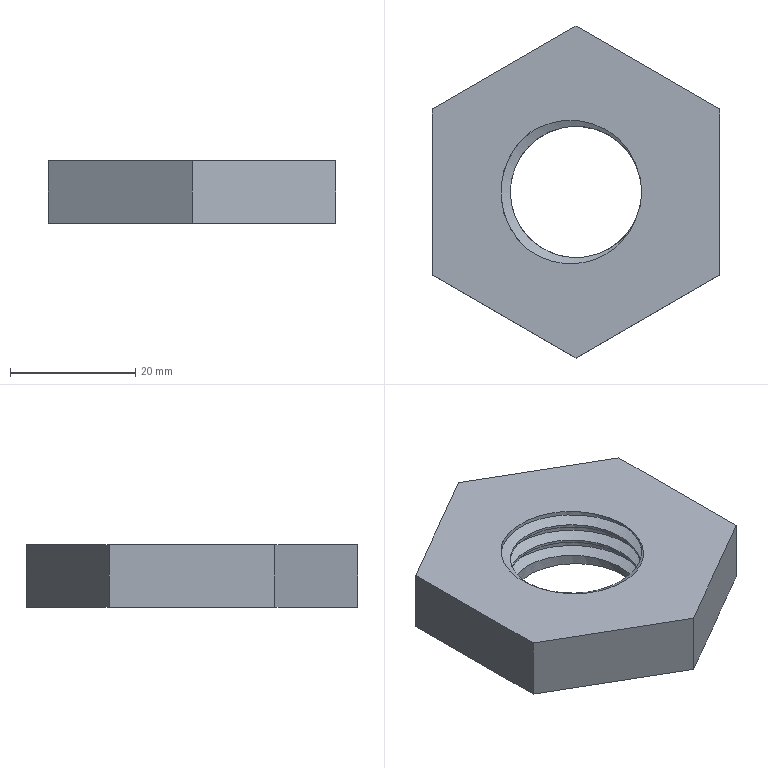Part | NX | features DATUM_CSYS 2, EXTRUDE 1, SKETCH 1, THREADS 1 | 1 solid | 13 faces | box 45.899 x 53 x 10 mm | volume 14258 mm3 | plane 9 | cylinder 2 | spline 2 | commonest cylinder face diameters 21 x1 24 x1
STEP:
#1=CARTESIAN_POINT('',(-9.733,-3.939,-10.));
#2=VERTEX_POINT('',#1);
#3=CARTESIAN_POINT('',(-9.733,-3.939,-7.535));
#4=VERTEX_POINT('',#3);
#5=CARTESIAN_POINT('',(-9.733,-3.939,-10.));
#6=DIRECTION('',(0.,0.,1.));
#7=VECTOR('',#6,1000.);
#8=LINE('',#5,#7);
#9=EDGE_CURVE('',#2,#4,#8,.T.);
#10=ORIENTED_EDGE('',*,*,#9,.F.);
#11=CARTESIAN_POINT('',(-8.724,-5.844,-10.));
#12=VERTEX_POINT('',#11);
#13=CARTESIAN_POINT('',(0.,0.,-10.));
#14=DIRECTION('',(0.,0.,1.));
#15=DIRECTION('',(1.,0.,0.));
#16=AXIS2_PLACEMENT_3D('',#13,#14,#15);
#17=CIRCLE('',#16,10.5);
#18=EDGE_CURVE('',#12,#2,#17,.T.);
#19=ORIENTED_EDGE('',*,*,#18,.F.);
#20=CARTESIAN_POINT('',(9.422,-4.634,0.));
#21=VERTEX_POINT('',#20);
#22=CARTESIAN_POINT('',(-8.724,-5.844,-10.));
#23=CARTESIAN_POINT('',(-7.437,-7.765,-9.895));
#24=CARTESIAN_POINT('',(-3.621,-10.672,-9.688));
#25=CARTESIAN_POINT('',(3.636,-10.678,-9.375));
#26=CARTESIAN_POINT('',(9.381,-6.256,-9.063));
#27=CARTESIAN_POINT('',(11.252,0.747,-8.75));
#28=CARTESIAN_POINT('',(8.472,7.443,-8.438));
#29=CARTESIAN_POINT('',(2.189,11.062,-8.125));
#30=CARTESIAN_POINT('',(-4.998,10.109,-7.813));
#31=CARTESIAN_POINT('',(-10.12,4.976,-7.5));
#32=CARTESIAN_POINT('',(-11.058,-2.214,-7.187));
#33=CARTESIAN_POINT('',(-7.424,-8.489,-6.875));
#34=CARTESIAN_POINT('',(-0.7214,-11.254,-6.562));
#35=CARTESIAN_POINT('',(6.279,-9.367,-6.25));
#36=CARTESIAN_POINT('',(10.684,-3.609,-5.937));
#37=CARTESIAN_POINT('',(10.673,3.64,-5.625));
#38=CARTESIAN_POINT('',(6.252,9.385,-5.312));
#39=CARTESIAN_POINT('',(-0.7512,11.251,-5.));
#40=CARTESIAN_POINT('',(-7.444,8.47,-4.688));
#41=CARTESIAN_POINT('',(-11.062,2.19,-4.375));
#42=CARTESIAN_POINT('',(-10.109,-4.996,-4.063));
#43=CARTESIAN_POINT('',(-4.979,-10.118,-3.75));
#44=CARTESIAN_POINT('',(2.21,-11.058,-3.438));
#45=CARTESIAN_POINT('',(8.486,-7.427,-3.125));
#46=CARTESIAN_POINT('',(11.254,-0.7254,-2.813));
#47=CARTESIAN_POINT('',(9.369,6.276,-2.5));
#48=CARTESIAN_POINT('',(3.611,10.683,-2.187));
#49=CARTESIAN_POINT('',(-3.64,10.673,-1.875));
#50=CARTESIAN_POINT('',(-9.386,6.251,-1.562));
#51=CARTESIAN_POINT('',(-11.252,-0.7548,-1.25));
#52=CARTESIAN_POINT('',(-8.467,-7.447,-0.9373));
#53=CARTESIAN_POINT('',(-2.185,-11.066,-0.625));
#54=CARTESIAN_POINT('',(5.007,-10.095,-0.3119));
#55=CARTESIAN_POINT('',(8.402,-6.709,-0.1051));
#56=CARTESIAN_POINT('',(9.422,-4.634,0.));
#57=B_SPLINE_CURVE_WITH_KNOTS('',3,(#22,#23,#24,#25,#26,#27,#28,#29,#30,#31,#32,#33,#34,#35,#36,#37,#38,#39,#40,#41,#42,#43,#44,#45,#46,#47,#48,#49,#50,#51,#52,#53,#54,#55,#56),.UNSPECIFIED.,.F.,.F.,(4,1,1,1,1,1,1,1,1,1,1,1,1,1,1,1,1,1,1,1,1,1,1,1,1,1,1,1,1,1,1,1,4),(0.,0.006847,0.01369,0.02054,0.02739,0.03423,0.04108,0.04793,0.05477,0.06162,0.06847,0.07531,0.08216,0.08901,0.09585,0.1027,0.1095,0.1164,0.1232,0.1301,0.1369,0.1438,0.1506,0.1575,0.1643,0.1712,0.178,0.1849,0.1917,0.1986,0.2054,0.2123,0.2191),.UNSPECIFIED.);
#58=EDGE_CURVE('',#12,#21,#57,.T.);
#59=ORIENTED_EDGE('',*,*,#58,.T.);
#60=CARTESIAN_POINT('',(9.422,4.634,0.));
#61=VERTEX_POINT('',#60);
#62=CARTESIAN_POINT('',(0.,0.,0.));
#63=DIRECTION('',(0.,0.,1.));
#64=DIRECTION('',(1.,0.,0.));
#65=AXIS2_PLACEMENT_3D('',#62,#63,#64);
#66=CIRCLE('',#65,10.5);
#67=EDGE_CURVE('',#21,#61,#66,.T.);
#68=ORIENTED_EDGE('',*,*,#67,.T.);
#69=CARTESIAN_POINT('',(9.422,4.634,0.));
#70=CARTESIAN_POINT('',(10.191,3.07,-0.07918));
#71=CARTESIAN_POINT('',(10.923,-0.3895,-0.2352));
#72=CARTESIAN_POINT('',(9.443,-5.518,-0.4707));
#73=CARTESIAN_POINT('',(5.696,-9.332,-0.7066));
#74=CARTESIAN_POINT('',(0.6132,-10.918,-0.9414));
#75=CARTESIAN_POINT('',(-4.642,-9.9,-1.178));
#76=CARTESIAN_POINT('',(-8.765,-6.537,-1.412));
#77=CARTESIAN_POINT('',(-10.818,-1.592,-1.648));
#78=CARTESIAN_POINT('',(-10.288,3.703,-1.883));
#79=CARTESIAN_POINT('',(-7.299,8.142,-2.119));
#80=CARTESIAN_POINT('',(-2.586,10.623,-2.354));
#81=CARTESIAN_POINT('',(2.759,10.581,-2.59));
#82=CARTESIAN_POINT('',(7.434,8.017,-2.825));
#83=CARTESIAN_POINT('',(10.345,3.543,-3.061));
#84=CARTESIAN_POINT('',(10.787,-1.78,-3.296));
#85=CARTESIAN_POINT('',(8.666,-6.668,-3.531));
#86=CARTESIAN_POINT('',(4.466,-9.98,-3.767));
#87=CARTESIAN_POINT('',(-0.7763,-10.907,-4.002));
#88=CARTESIAN_POINT('',(-5.86,-9.231,-4.238));
#89=CARTESIAN_POINT('',(-9.524,-5.372,-4.473));
#90=CARTESIAN_POINT('',(-10.932,-0.2071,-4.709));
#91=CARTESIAN_POINT('',(-9.735,4.979,-4.944));
#92=CARTESIAN_POINT('',(-6.207,9.002,-5.18));
#93=CARTESIAN_POINT('',(-1.217,10.865,-5.415));
#94=CARTESIAN_POINT('',(4.078,10.146,-5.651));
#95=CARTESIAN_POINT('',(8.392,7.008,-5.886));
#96=CARTESIAN_POINT('',(10.711,2.203,-6.121));
#97=CARTESIAN_POINT('',(10.474,-3.135,-6.357));
#98=CARTESIAN_POINT('',(7.751,-7.713,-6.592));
#99=CARTESIAN_POINT('',(3.163,-10.466,-6.828));
#100=CARTESIAN_POINT('',(-2.153,-10.721,-7.063));
#101=CARTESIAN_POINT('',(-6.984,-8.412,-7.299));
#102=CARTESIAN_POINT('',(-9.08,-5.554,-7.455));
#103=CARTESIAN_POINT('',(-9.733,-3.939,-7.535));
#104=B_SPLINE_CURVE_WITH_KNOTS('',3,(#69,#70,#71,#72,#73,#74,#75,#76,#77,#78,#79,#80,#81,#82,#83,#84,#85,#86,#87,#88,#89,#90,#91,#92,#93,#94,#95,#96,#97,#98,#99,#100,#101,#102,#103),.UNSPECIFIED.,.F.,.F.,(4,1,1,1,1,1,1,1,1,1,1,1,1,1,1,1,1,1,1,1,1,1,1,1,1,1,1,1,1,1,1,1,4),(0.,0.005158,0.01032,0.01548,0.02063,0.02579,0.03095,0.03611,0.04127,0.04643,0.05158,0.05674,0.0619,0.06706,0.07222,0.07738,0.08253,0.08769,0.09285,0.09801,0.1032,0.1083,0.1135,0.1186,0.1238,0.129,0.1341,0.1393,0.1444,0.1496,0.1548,0.1599,0.1651),.UNSPECIFIED.);
#105=EDGE_CURVE('',#61,#4,#104,.T.);
#106=ORIENTED_EDGE('',*,*,#105,.T.);
#107=EDGE_LOOP('',(#10,#19,#59,#68,#106));
#108=FACE_BOUND('',#107,.T.);
#109=CARTESIAN_POINT('',(0.,0.,-10.));
#110=DIRECTION('',(0.,0.,1.));
#111=DIRECTION('',(1.,0.,0.));
#112=AXIS2_PLACEMENT_3D('',#109,#110,#111);
#113=CYLINDRICAL_SURFACE('',#112,10.5);
#114=ADVANCED_FACE('',(#108),#113,.F.);
#115=CARTESIAN_POINT('',(-22.95,13.25,-10.));
#116=VERTEX_POINT('',#115);
#117=CARTESIAN_POINT('',(-22.95,-13.25,-10.));
#118=VERTEX_POINT('',#117);
#119=CARTESIAN_POINT('',(-22.95,13.25,-10.));
#120=DIRECTION('',(0.,-1.,0.));
#121=VECTOR('',#120,1000.);
#122=LINE('',#119,#121);
#123=EDGE_CURVE('',#116,#118,#122,.T.);
#124=ORIENTED_EDGE('',*,*,#123,.F.);
#125=CARTESIAN_POINT('',(0.,26.5,-10.));
#126=VERTEX_POINT('',#125);
#127=CARTESIAN_POINT('',(0.,26.5,-10.));
#128=DIRECTION('',(-0.866,-0.5,0.));
#129=VECTOR('',#128,1000.);
#130=LINE('',#127,#129);
#131=EDGE_CURVE('',#126,#116,#130,.T.);
#132=ORIENTED_EDGE('',*,*,#131,.F.);
#133=CARTESIAN_POINT('',(22.95,13.25,-10.));
#134=VERTEX_POINT('',#133);
#135=CARTESIAN_POINT('',(22.95,13.25,-10.));
#136=DIRECTION('',(-0.866,0.5,0.));
#137=VECTOR('',#136,1000.);
#138=LINE('',#135,#137);
#139=EDGE_CURVE('',#134,#126,#138,.T.);
#140=ORIENTED_EDGE('',*,*,#139,.F.);
#141=CARTESIAN_POINT('',(22.95,-13.25,-10.));
#142=VERTEX_POINT('',#141);
#143=CARTESIAN_POINT('',(22.95,-13.25,-10.));
#144=DIRECTION('',(0.,1.,0.));
#145=VECTOR('',#144,1000.);
#146=LINE('',#143,#145);
#147=EDGE_CURVE('',#142,#134,#146,.T.);
#148=ORIENTED_EDGE('',*,*,#147,.F.);
#149=CARTESIAN_POINT('',(0.,-26.5,-10.));
#150=VERTEX_POINT('',#149);
#151=CARTESIAN_POINT('',(0.,-26.5,-10.));
#152=DIRECTION('',(0.866,0.5,0.));
#153=VECTOR('',#152,1000.);
#154=LINE('',#151,#153);
#155=EDGE_CURVE('',#150,#142,#154,.T.);
#156=ORIENTED_EDGE('',*,*,#155,.F.);
#157=CARTESIAN_POINT('',(-22.95,-13.25,-10.));
#158=DIRECTION('',(0.866,-0.5,0.));
#159=VECTOR('',#158,1000.);
#160=LINE('',#157,#159);
#161=EDGE_CURVE('',#118,#150,#160,.T.);
#162=ORIENTED_EDGE('',*,*,#161,.F.);
#163=EDGE_LOOP('',(#124,#132,#140,#148,#156,#162));
#164=FACE_BOUND('',#163,.T.);
#165=CARTESIAN_POINT('',(-9.891,-4.002,-10.));
#166=VERTEX_POINT('',#165);
#167=CARTESIAN_POINT('',(0.,0.,-10.));
#168=DIRECTION('',(0.927,0.3751,0.));
#169=VECTOR('',#168,1000.);
#170=LINE('',#167,#169);
#171=EDGE_CURVE('',#166,#2,#170,.T.);
#172=ORIENTED_EDGE('',*,*,#171,.F.);
#173=CARTESIAN_POINT('',(-9.891,-4.002,-10.));
#174=CARTESIAN_POINT('',(-9.565,-4.657,-10.));
#175=CARTESIAN_POINT('',(-9.176,-5.271,-10.));
#176=CARTESIAN_POINT('',(-8.724,-5.844,-10.));
#177=B_SPLINE_CURVE_WITH_KNOTS('',3,(#173,#174,#175,#176),.UNSPECIFIED.,.F.,.F.,(4,4),(0.,0.00218),.UNSPECIFIED.);
#178=EDGE_CURVE('',#166,#12,#177,.T.);
#179=ORIENTED_EDGE('',*,*,#178,.T.);
#180=ORIENTED_EDGE('',*,*,#18,.T.);
#181=EDGE_LOOP('',(#172,#179,#180));
#182=FACE_BOUND('',#181,.T.);
#183=CARTESIAN_POINT('',(0.,0.,-10.));
#184=DIRECTION('',(0.,0.,1.));
#185=DIRECTION('',(1.,0.,0.));
#186=AXIS2_PLACEMENT_3D('',#183,#184,#185);
#187=PLANE('',#186);
#188=ADVANCED_FACE('',(#164,#182),#187,.F.);
#189=CARTESIAN_POINT('',(-22.95,13.25,0.));
#190=VERTEX_POINT('',#189);
#191=CARTESIAN_POINT('',(-22.95,-13.25,0.));
#192=VERTEX_POINT('',#191);
#193=CARTESIAN_POINT('',(-22.95,13.25,0.));
#194=DIRECTION('',(0.,-1.,0.));
#195=VECTOR('',#194,1000.);
#196=LINE('',#193,#195);
#197=EDGE_CURVE('',#190,#192,#196,.T.);
#198=ORIENTED_EDGE('',*,*,#197,.F.);
#199=CARTESIAN_POINT('',(-22.95,13.25,-10.));
#200=DIRECTION('',(0.,0.,1.));
#201=VECTOR('',#200,1000.);
#202=LINE('',#199,#201);
#203=EDGE_CURVE('',#116,#190,#202,.T.);
#204=ORIENTED_EDGE('',*,*,#203,.F.);
#205=ORIENTED_EDGE('',*,*,#123,.T.);
#206=CARTESIAN_POINT('',(-22.95,-13.25,-10.));
#207=DIRECTION('',(0.,0.,1.));
#208=VECTOR('',#207,1000.);
#209=LINE('',#206,#208);
#210=EDGE_CURVE('',#118,#192,#209,.T.);
#211=ORIENTED_EDGE('',*,*,#210,.T.);
#212=EDGE_LOOP('',(#198,#204,#205,#211));
#213=FACE_BOUND('',#212,.T.);
#214=CARTESIAN_POINT('',(-22.95,13.25,-10.));
#215=DIRECTION('',(-1.,0.,0.));
#216=DIRECTION('',(0.,-1.,0.));
#217=AXIS2_PLACEMENT_3D('',#214,#215,#216);
#218=PLANE('',#217);
#219=ADVANCED_FACE('',(#213),#218,.T.);
#220=CARTESIAN_POINT('',(0.,-26.5,0.));
#221=VERTEX_POINT('',#220);
#222=CARTESIAN_POINT('',(-22.95,-13.25,0.));
#223=DIRECTION('',(0.866,-0.5,0.));
#224=VECTOR('',#223,1000.);
#225=LINE('',#222,#224);
#226=EDGE_CURVE('',#192,#221,#225,.T.);
#227=ORIENTED_EDGE('',*,*,#226,.F.);
#228=ORIENTED_EDGE('',*,*,#210,.F.);
#229=ORIENTED_EDGE('',*,*,#161,.T.);
#230=CARTESIAN_POINT('',(0.,-26.5,-10.));
#231=DIRECTION('',(0.,0.,1.));
#232=VECTOR('',#231,1000.);
#233=LINE('',#230,#232);
#234=EDGE_CURVE('',#150,#221,#233,.T.);
#235=ORIENTED_EDGE('',*,*,#234,.T.);
#236=EDGE_LOOP('',(#227,#228,#229,#235));
#237=FACE_BOUND('',#236,.T.);
#238=CARTESIAN_POINT('',(-22.95,-13.25,-10.));
#239=DIRECTION('',(-0.5,-0.866,0.));
#240=DIRECTION('',(0.866,-0.5,0.));
#241=AXIS2_PLACEMENT_3D('',#238,#239,#240);
#242=PLANE('',#241);
#243=ADVANCED_FACE('',(#237),#242,.T.);
#244=CARTESIAN_POINT('',(22.95,-13.25,0.));
#245=VERTEX_POINT('',#244);
#246=CARTESIAN_POINT('',(0.,-26.5,0.));
#247=DIRECTION('',(0.866,0.5,0.));
#248=VECTOR('',#247,1000.);
#249=LINE('',#246,#248);
#250=EDGE_CURVE('',#221,#245,#249,.T.);
#251=ORIENTED_EDGE('',*,*,#250,.F.);
#252=ORIENTED_EDGE('',*,*,#234,.F.);
#253=ORIENTED_EDGE('',*,*,#155,.T.);
#254=CARTESIAN_POINT('',(22.95,-13.25,-10.));
#255=DIRECTION('',(0.,0.,1.));
#256=VECTOR('',#255,1000.);
#257=LINE('',#254,#256);
#258=EDGE_CURVE('',#142,#245,#257,.T.);
#259=ORIENTED_EDGE('',*,*,#258,.T.);
#260=EDGE_LOOP('',(#251,#252,#253,#259));
#261=FACE_BOUND('',#260,.T.);
#262=CARTESIAN_POINT('',(0.,-26.5,-10.));
#263=DIRECTION('',(0.5,-0.866,0.));
#264=DIRECTION('',(0.866,0.5,0.));
#265=AXIS2_PLACEMENT_3D('',#262,#263,#264);
#266=PLANE('',#265);
#267=ADVANCED_FACE('',(#261),#266,.T.);
#268=CARTESIAN_POINT('',(22.95,13.25,0.));
#269=VERTEX_POINT('',#268);
#270=CARTESIAN_POINT('',(22.95,-13.25,0.));
#271=DIRECTION('',(0.,1.,0.));
#272=VECTOR('',#271,1000.);
#273=LINE('',#270,#272);
#274=EDGE_CURVE('',#245,#269,#273,.T.);
#275=ORIENTED_EDGE('',*,*,#274,.F.);
#276=ORIENTED_EDGE('',*,*,#258,.F.);
#277=ORIENTED_EDGE('',*,*,#147,.T.);
#278=CARTESIAN_POINT('',(22.95,13.25,-10.));
#279=DIRECTION('',(0.,0.,1.));
#280=VECTOR('',#279,1000.);
#281=LINE('',#278,#280);
#282=EDGE_CURVE('',#134,#269,#281,.T.);
#283=ORIENTED_EDGE('',*,*,#282,.T.);
#284=EDGE_LOOP('',(#275,#276,#277,#283));
#285=FACE_BOUND('',#284,.T.);
#286=CARTESIAN_POINT('',(22.95,-13.25,-10.));
#287=DIRECTION('',(1.,0.,0.));
#288=DIRECTION('',(0.,0.,-1.));
#289=AXIS2_PLACEMENT_3D('',#286,#287,#288);
#290=PLANE('',#289);
#291=ADVANCED_FACE('',(#285),#290,.T.);
#292=CARTESIAN_POINT('',(0.,26.5,0.));
#293=VERTEX_POINT('',#292);
#294=CARTESIAN_POINT('',(22.95,13.25,0.));
#295=DIRECTION('',(-0.866,0.5,0.));
#296=VECTOR('',#295,1000.);
#297=LINE('',#294,#296);
#298=EDGE_CURVE('',#269,#293,#297,.T.);
#299=ORIENTED_EDGE('',*,*,#298,.F.);
#300=ORIENTED_EDGE('',*,*,#282,.F.);
#301=ORIENTED_EDGE('',*,*,#139,.T.);
#302=CARTESIAN_POINT('',(0.,26.5,-10.));
#303=DIRECTION('',(0.,0.,1.));
#304=VECTOR('',#303,1000.);
#305=LINE('',#302,#304);
#306=EDGE_CURVE('',#126,#293,#305,.T.);
#307=ORIENTED_EDGE('',*,*,#306,.T.);
#308=EDGE_LOOP('',(#299,#300,#301,#307));
#309=FACE_BOUND('',#308,.T.);
#310=CARTESIAN_POINT('',(22.95,13.25,-10.));
#311=DIRECTION('',(0.5,0.866,0.));
#312=DIRECTION('',(-0.866,0.5,0.));
#313=AXIS2_PLACEMENT_3D('',#310,#311,#312);
#314=PLANE('',#313);
#315=ADVANCED_FACE('',(#309),#314,.T.);
#316=CARTESIAN_POINT('',(0.,26.5,0.));
#317=DIRECTION('',(-0.866,-0.5,0.));
#318=VECTOR('',#317,1000.);
#319=LINE('',#316,#318);
#320=EDGE_CURVE('',#293,#190,#319,.T.);
#321=ORIENTED_EDGE('',*,*,#320,.F.);
#322=ORIENTED_EDGE('',*,*,#306,.F.);
#323=ORIENTED_EDGE('',*,*,#131,.T.);
#324=ORIENTED_EDGE('',*,*,#203,.T.);
#325=EDGE_LOOP('',(#321,#322,#323,#324));
#326=FACE_BOUND('',#325,.T.);
#327=CARTESIAN_POINT('',(0.,26.5,-10.));
#328=DIRECTION('',(-0.5,0.866,0.));
#329=DIRECTION('',(-0.866,-0.5,0.));
#330=AXIS2_PLACEMENT_3D('',#327,#328,#329);
#331=PLANE('',#330);
#332=ADVANCED_FACE('',(#326),#331,.T.);
#333=CARTESIAN_POINT('',(-7.731,9.178,0.));
#334=VERTEX_POINT('',#333);
#335=CARTESIAN_POINT('',(9.422,4.634,0.));
#336=CARTESIAN_POINT('',(8.153,7.825,0.));
#337=CARTESIAN_POINT('',(3.85,11.452,0.));
#338=CARTESIAN_POINT('',(-3.166,11.596,0.));
#339=CARTESIAN_POINT('',(-6.345,10.191,0.));
#340=CARTESIAN_POINT('',(-7.731,9.178,0.));
#341=B_SPLINE_CURVE_WITH_KNOTS('',3,(#335,#336,#337,#338,#339,#340),.UNSPECIFIED.,.F.,.F.,(4,1,1,4),(0.000126,0.0103,0.01539,0.02048),.UNSPECIFIED.);
#342=EDGE_CURVE('',#61,#334,#341,.T.);
#343=ORIENTED_EDGE('',*,*,#342,.F.);
#344=ORIENTED_EDGE('',*,*,#67,.F.);
#345=CARTESIAN_POINT('',(-7.731,-9.178,0.));
#346=VERTEX_POINT('',#345);
#347=CARTESIAN_POINT('',(-7.731,-9.178,0.));
#348=CARTESIAN_POINT('',(-6.345,-10.191,0.));
#349=CARTESIAN_POINT('',(-3.169,-11.593,0.));
#350=CARTESIAN_POINT('',(3.824,-11.46,0.));
#351=CARTESIAN_POINT('',(8.15,-7.833,0.));
#352=CARTESIAN_POINT('',(9.422,-4.634,0.));
#353=B_SPLINE_CURVE_WITH_KNOTS('',3,(#347,#348,#349,#350,#351,#352),.UNSPECIFIED.,.F.,.F.,(4,1,1,4),(0.000131,0.005219,0.01031,0.02048),.UNSPECIFIED.);
#354=EDGE_CURVE('',#346,#21,#353,.T.);
#355=ORIENTED_EDGE('',*,*,#354,.F.);
#356=CARTESIAN_POINT('',(0.,0.,0.));
#357=DIRECTION('',(0.,0.,-1.));
#358=DIRECTION('',(-1.,0.,0.));
#359=AXIS2_PLACEMENT_3D('',#356,#357,#358);
#360=CIRCLE('',#359,12.);
#361=EDGE_CURVE('',#334,#346,#360,.F.);
#362=ORIENTED_EDGE('',*,*,#361,.F.);
#363=EDGE_LOOP('',(#343,#344,#355,#362));
#364=FACE_BOUND('',#363,.T.);
#365=ORIENTED_EDGE('',*,*,#197,.T.);
#366=ORIENTED_EDGE('',*,*,#226,.T.);
#367=ORIENTED_EDGE('',*,*,#250,.T.);
#368=ORIENTED_EDGE('',*,*,#274,.T.);
#369=ORIENTED_EDGE('',*,*,#298,.T.);
#370=ORIENTED_EDGE('',*,*,#320,.T.);
#371=EDGE_LOOP('',(#365,#366,#367,#368,#369,#370));
#372=FACE_BOUND('',#371,.T.);
#373=CARTESIAN_POINT('',(0.,0.,0.));
#374=DIRECTION('',(0.,0.,1.));
#375=DIRECTION('',(1.,0.,0.));
#376=AXIS2_PLACEMENT_3D('',#373,#374,#375);
#377=PLANE('',#376);
#378=ADVANCED_FACE('',(#364,#372),#377,.T.);
#379=ORIENTED_EDGE('',*,*,#342,.T.);
#380=CARTESIAN_POINT('',(-11.124,-4.501,-8.401));
#381=VERTEX_POINT('',#380);
#382=CARTESIAN_POINT('',(-11.124,-4.501,-8.401));
#383=CARTESIAN_POINT('',(-10.291,-6.559,-8.312));
#384=CARTESIAN_POINT('',(-7.51,-10.137,-8.139));
#385=CARTESIAN_POINT('',(-1.083,-12.576,-7.875));
#386=CARTESIAN_POINT('',(5.631,-11.291,-7.613));
#387=CARTESIAN_POINT('',(10.709,-6.682,-7.351));
#388=CARTESIAN_POINT('',(12.618,-0.09366,-7.088));
#389=CARTESIAN_POINT('',(10.816,6.5,-6.826));
#390=CARTESIAN_POINT('',(5.815,11.202,-6.563));
#391=CARTESIAN_POINT('',(-0.8925,12.586,-6.3));
#392=CARTESIAN_POINT('',(-7.333,10.273,-6.038));
#393=CARTESIAN_POINT('',(-11.625,4.913,-5.775));
#394=CARTESIAN_POINT('',(-12.479,-1.871,-5.513));
#395=CARTESIAN_POINT('',(-9.663,-8.121,-5.251));
#396=CARTESIAN_POINT('',(-3.984,-11.973,-4.988));
#397=CARTESIAN_POINT('',(2.843,-12.295,-4.726));
#398=CARTESIAN_POINT('',(8.859,-8.991,-4.463));
#399=CARTESIAN_POINT('',(12.247,-3.035,-4.2));
#400=CARTESIAN_POINT('',(12.034,3.802,-3.938));
#401=CARTESIAN_POINT('',(8.263,9.54,-3.675));
#402=CARTESIAN_POINT('',(2.071,12.447,-3.413));
#403=CARTESIAN_POINT('',(-4.74,11.698,-3.15));
#404=CARTESIAN_POINT('',(-10.159,7.486,-2.887));
#405=CARTESIAN_POINT('',(-12.572,1.091,-2.626));
#406=CARTESIAN_POINT('',(-11.288,-5.649,-2.363));
#407=CARTESIAN_POINT('',(-6.667,-10.713,-2.1));
#408=CARTESIAN_POINT('',(-0.1,-12.62,-1.838));
#409=CARTESIAN_POINT('',(6.522,-10.805,-1.575));
#410=CARTESIAN_POINT('',(11.2,-5.812,-1.313));
#411=CARTESIAN_POINT('',(12.59,0.8957,-1.05));
#412=CARTESIAN_POINT('',(10.257,7.351,-0.7873));
#413=CARTESIAN_POINT('',(4.92,11.621,-0.5255));
#414=CARTESIAN_POINT('',(-1.891,12.477,-0.2624));
#415=CARTESIAN_POINT('',(-6.042,10.6,-0.08788));
#416=CARTESIAN_POINT('',(-7.731,9.178,0.));
#417=B_SPLINE_CURVE_WITH_KNOTS('',3,(#382,#383,#384,#385,#386,#387,#388,#389,#390,#391,#392,#393,#394,#395,#396,#397,#398,#399,#400,#401,#402,#403,#404,#405,#406,#407,#408,#409,#410,#411,#412,#413,#414,#415,#416),.UNSPECIFIED.,.F.,.F.,(4,1,1,1,1,1,1,1,1,1,1,1,1,1,1,1,1,1,1,1,1,1,1,1,1,1,1,1,1,1,1,1,4),(0.,0.006572,0.01314,0.01972,0.02629,0.03286,0.03943,0.046,0.05257,0.05915,0.06572,0.07229,0.07886,0.08543,0.092,0.09858,0.1051,0.1117,0.1183,0.1249,0.1314,0.138,0.1446,0.1511,0.1577,0.1643,0.1709,0.1774,0.184,0.1906,0.1972,0.2037,0.2103),.UNSPECIFIED.);
#418=EDGE_CURVE('',#334,#381,#417,.F.);
#419=ORIENTED_EDGE('',*,*,#418,.T.);
#420=CARTESIAN_POINT('',(-11.582,-4.687,-8.686));
#421=CARTESIAN_POINT('',(-9.724,-3.935,-7.529));
#422=B_SPLINE_CURVE_WITH_KNOTS('',1,(#420,#421),.UNSPECIFIED.,.F.,.F.,(2,2),(0.,1.),.PIECEWISE_BEZIER_KNOTS.);
#423=EDGE_CURVE('',#381,#4,#422,.T.);
#424=ORIENTED_EDGE('',*,*,#423,.T.);
#425=ORIENTED_EDGE('',*,*,#105,.F.);
#426=EDGE_LOOP('',(#379,#419,#424,#425));
#427=FACE_BOUND('',#426,.T.);
#428=CARTESIAN_POINT('',(-8.662,8.318,0.0452));
#429=CARTESIAN_POINT('',(-8.606,8.377,0.04198));
#430=CARTESIAN_POINT('',(-7.999,8.996,0.007513));
#431=CARTESIAN_POINT('',(-6.715,10.05,-0.05821));
#432=CARTESIAN_POINT('',(-4.625,11.166,-0.152));
#433=CARTESIAN_POINT('',(-2.358,11.854,-0.2457));
#434=CARTESIAN_POINT('',(0.,12.086,-0.3395));
#435=CARTESIAN_POINT('',(2.358,11.854,-0.4332));
#436=CARTESIAN_POINT('',(4.625,11.166,-0.527));
#437=CARTESIAN_POINT('',(6.715,10.05,-0.6207));
#438=CARTESIAN_POINT('',(8.546,8.546,-0.7145));
#439=CARTESIAN_POINT('',(10.05,6.715,-0.8082));
#440=CARTESIAN_POINT('',(11.166,4.625,-0.902));
#441=CARTESIAN_POINT('',(11.854,2.358,-0.9957));
#442=CARTESIAN_POINT('',(12.086,0.,-1.089));
#443=CARTESIAN_POINT('',(11.854,-2.358,-1.183));
#444=CARTESIAN_POINT('',(11.166,-4.625,-1.277));
#445=CARTESIAN_POINT('',(10.05,-6.715,-1.371));
#446=CARTESIAN_POINT('',(8.546,-8.546,-1.464));
#447=CARTESIAN_POINT('',(6.715,-10.05,-1.558));
#448=CARTESIAN_POINT('',(4.625,-11.166,-1.652));
#449=CARTESIAN_POINT('',(2.358,-11.854,-1.746));
#450=CARTESIAN_POINT('',(0.,-12.086,-1.839));
#451=CARTESIAN_POINT('',(-2.358,-11.854,-1.933));
#452=CARTESIAN_POINT('',(-4.625,-11.166,-2.027));
#453=CARTESIAN_POINT('',(-6.715,-10.05,-2.121));
#454=CARTESIAN_POINT('',(-8.546,-8.546,-2.214));
#455=CARTESIAN_POINT('',(-10.05,-6.715,-2.308));
#456=CARTESIAN_POINT('',(-11.166,-4.625,-2.402));
#457=CARTESIAN_POINT('',(-11.854,-2.358,-2.496));
#458=CARTESIAN_POINT('',(-12.086,0.,-2.589));
#459=CARTESIAN_POINT('',(-11.854,2.358,-2.683));
#460=CARTESIAN_POINT('',(-11.166,4.625,-2.777));
#461=CARTESIAN_POINT('',(-10.05,6.715,-2.871));
#462=CARTESIAN_POINT('',(-8.546,8.546,-2.964));
#463=CARTESIAN_POINT('',(-6.715,10.05,-3.058));
#464=CARTESIAN_POINT('',(-4.625,11.166,-3.152));
#465=CARTESIAN_POINT('',(-2.358,11.854,-3.246));
#466=CARTESIAN_POINT('',(0.,12.086,-3.339));
#467=CARTESIAN_POINT('',(2.358,11.854,-3.433));
#468=CARTESIAN_POINT('',(4.625,11.166,-3.527));
#469=CARTESIAN_POINT('',(6.715,10.05,-3.621));
#470=CARTESIAN_POINT('',(8.546,8.546,-3.714));
#471=CARTESIAN_POINT('',(10.05,6.715,-3.808));
#472=CARTESIAN_POINT('',(11.166,4.625,-3.902));
#473=CARTESIAN_POINT('',(11.854,2.358,-3.996));
#474=CARTESIAN_POINT('',(12.086,0.,-4.089));
#475=CARTESIAN_POINT('',(11.854,-2.358,-4.183));
#476=CARTESIAN_POINT('',(11.166,-4.625,-4.277));
#477=CARTESIAN_POINT('',(10.05,-6.715,-4.371));
#478=CARTESIAN_POINT('',(8.546,-8.546,-4.464));
#479=CARTESIAN_POINT('',(6.715,-10.05,-4.558));
#480=CARTESIAN_POINT('',(4.625,-11.166,-4.652));
#481=CARTESIAN_POINT('',(2.358,-11.854,-4.746));
#482=CARTESIAN_POINT('',(0.,-12.086,-4.839));
#483=CARTESIAN_POINT('',(-2.358,-11.854,-4.933));
#484=CARTESIAN_POINT('',(-4.625,-11.166,-5.027));
#485=CARTESIAN_POINT('',(-6.715,-10.05,-5.121));
#486=CARTESIAN_POINT('',(-8.546,-8.546,-5.214));
#487=CARTESIAN_POINT('',(-10.05,-6.715,-5.308));
#488=CARTESIAN_POINT('',(-11.166,-4.625,-5.402));
#489=CARTESIAN_POINT('',(-11.854,-2.358,-5.496));
#490=CARTESIAN_POINT('',(-12.086,0.,-5.589));
#491=CARTESIAN_POINT('',(-11.854,2.358,-5.683));
#492=CARTESIAN_POINT('',(-11.166,4.625,-5.777));
#493=CARTESIAN_POINT('',(-10.05,6.715,-5.871));
#494=CARTESIAN_POINT('',(-8.546,8.546,-5.964));
#495=CARTESIAN_POINT('',(-6.715,10.05,-6.058));
#496=CARTESIAN_POINT('',(-4.625,11.166,-6.152));
#497=CARTESIAN_POINT('',(-2.358,11.854,-6.246));
#498=CARTESIAN_POINT('',(0.,12.086,-6.339));
#499=CARTESIAN_POINT('',(2.358,11.854,-6.433));
#500=CARTESIAN_POINT('',(4.625,11.166,-6.527));
#501=CARTESIAN_POINT('',(6.715,10.05,-6.621));
#502=CARTESIAN_POINT('',(8.546,8.546,-6.714));
#503=CARTESIAN_POINT('',(10.05,6.715,-6.808));
#504=CARTESIAN_POINT('',(11.166,4.625,-6.902));
#505=CARTESIAN_POINT('',(11.854,2.358,-6.996));
#506=CARTESIAN_POINT('',(12.086,0.,-7.089));
#507=CARTESIAN_POINT('',(11.854,-2.358,-7.183));
#508=CARTESIAN_POINT('',(11.166,-4.625,-7.277));
#509=CARTESIAN_POINT('',(10.05,-6.715,-7.371));
#510=CARTESIAN_POINT('',(8.546,-8.546,-7.464));
#511=CARTESIAN_POINT('',(6.715,-10.05,-7.558));
#512=CARTESIAN_POINT('',(4.625,-11.166,-7.652));
#513=CARTESIAN_POINT('',(2.358,-11.854,-7.746));
#514=CARTESIAN_POINT('',(0.,-12.086,-7.839));
#515=CARTESIAN_POINT('',(-2.358,-11.854,-7.933));
#516=CARTESIAN_POINT('',(-4.625,-11.166,-8.027));
#517=CARTESIAN_POINT('',(-6.715,-10.05,-8.121));
#518=CARTESIAN_POINT('',(-8.546,-8.546,-8.214));
#519=CARTESIAN_POINT('',(-10.05,-6.715,-8.308));
#520=CARTESIAN_POINT('',(-10.81,-5.293,-8.372));
#521=CARTESIAN_POINT('',(-11.12,-4.535,-8.405));
#522=CARTESIAN_POINT('',(-11.132,-4.505,-8.406));
#523=CARTESIAN_POINT('',(-7.567,7.267,0.9217));
#524=CARTESIAN_POINT('',(-7.518,7.318,0.9185));
#525=CARTESIAN_POINT('',(-6.988,7.859,0.884));
#526=CARTESIAN_POINT('',(-5.866,8.779,0.8183));
#527=CARTESIAN_POINT('',(-4.041,9.755,0.7245));
#528=CARTESIAN_POINT('',(-2.06,10.356,0.6308));
#529=CARTESIAN_POINT('',(0.,10.559,0.537));
#530=CARTESIAN_POINT('',(2.06,10.356,0.4433));
#531=CARTESIAN_POINT('',(4.041,9.755,0.3495));
#532=CARTESIAN_POINT('',(5.866,8.779,0.2558));
#533=CARTESIAN_POINT('',(7.466,7.466,0.162));
#534=CARTESIAN_POINT('',(8.779,5.866,0.06828));
#535=CARTESIAN_POINT('',(9.755,4.041,-0.02547));
#536=CARTESIAN_POINT('',(10.356,2.06,-0.1192));
#537=CARTESIAN_POINT('',(10.559,0.,-0.213));
#538=CARTESIAN_POINT('',(10.356,-2.06,-0.3067));
#539=CARTESIAN_POINT('',(9.755,-4.041,-0.4005));
#540=CARTESIAN_POINT('',(8.779,-5.866,-0.4942));
#541=CARTESIAN_POINT('',(7.466,-7.466,-0.588));
#542=CARTESIAN_POINT('',(5.866,-8.779,-0.6817));
#543=CARTESIAN_POINT('',(4.041,-9.755,-0.7755));
#544=CARTESIAN_POINT('',(2.06,-10.356,-0.8692));
#545=CARTESIAN_POINT('',(0.,-10.559,-0.963));
#546=CARTESIAN_POINT('',(-2.06,-10.356,-1.057));
#547=CARTESIAN_POINT('',(-4.041,-9.755,-1.15));
#548=CARTESIAN_POINT('',(-5.866,-8.779,-1.244));
#549=CARTESIAN_POINT('',(-7.466,-7.466,-1.338));
#550=CARTESIAN_POINT('',(-8.779,-5.866,-1.432));
#551=CARTESIAN_POINT('',(-9.755,-4.041,-1.525));
#552=CARTESIAN_POINT('',(-10.356,-2.06,-1.619));
#553=CARTESIAN_POINT('',(-10.559,0.,-1.713));
#554=CARTESIAN_POINT('',(-10.356,2.06,-1.807));
#555=CARTESIAN_POINT('',(-9.755,4.041,-1.9));
#556=CARTESIAN_POINT('',(-8.779,5.866,-1.994));
#557=CARTESIAN_POINT('',(-7.466,7.466,-2.088));
#558=CARTESIAN_POINT('',(-5.866,8.779,-2.182));
#559=CARTESIAN_POINT('',(-4.041,9.755,-2.275));
#560=CARTESIAN_POINT('',(-2.06,10.356,-2.369));
#561=CARTESIAN_POINT('',(0.,10.559,-2.463));
#562=CARTESIAN_POINT('',(2.06,10.356,-2.557));
#563=CARTESIAN_POINT('',(4.041,9.755,-2.65));
#564=CARTESIAN_POINT('',(5.866,8.779,-2.744));
#565=CARTESIAN_POINT('',(7.466,7.466,-2.838));
#566=CARTESIAN_POINT('',(8.779,5.866,-2.932));
#567=CARTESIAN_POINT('',(9.755,4.041,-3.025));
#568=CARTESIAN_POINT('',(10.356,2.06,-3.119));
#569=CARTESIAN_POINT('',(10.559,0.,-3.213));
#570=CARTESIAN_POINT('',(10.356,-2.06,-3.307));
#571=CARTESIAN_POINT('',(9.755,-4.041,-3.4));
#572=CARTESIAN_POINT('',(8.779,-5.866,-3.494));
#573=CARTESIAN_POINT('',(7.466,-7.466,-3.588));
#574=CARTESIAN_POINT('',(5.866,-8.779,-3.682));
#575=CARTESIAN_POINT('',(4.041,-9.755,-3.775));
#576=CARTESIAN_POINT('',(2.06,-10.356,-3.869));
#577=CARTESIAN_POINT('',(0.,-10.559,-3.963));
#578=CARTESIAN_POINT('',(-2.06,-10.356,-4.057));
#579=CARTESIAN_POINT('',(-4.041,-9.755,-4.15));
#580=CARTESIAN_POINT('',(-5.866,-8.779,-4.244));
#581=CARTESIAN_POINT('',(-7.466,-7.466,-4.338));
#582=CARTESIAN_POINT('',(-8.779,-5.866,-4.432));
#583=CARTESIAN_POINT('',(-9.755,-4.041,-4.525));
#584=CARTESIAN_POINT('',(-10.356,-2.06,-4.619));
#585=CARTESIAN_POINT('',(-10.559,0.,-4.713));
#586=CARTESIAN_POINT('',(-10.356,2.06,-4.807));
#587=CARTESIAN_POINT('',(-9.755,4.041,-4.9));
#588=CARTESIAN_POINT('',(-8.779,5.866,-4.994));
#589=CARTESIAN_POINT('',(-7.466,7.466,-5.088));
#590=CARTESIAN_POINT('',(-5.866,8.779,-5.182));
#591=CARTESIAN_POINT('',(-4.041,9.755,-5.275));
#592=CARTESIAN_POINT('',(-2.06,10.356,-5.369));
#593=CARTESIAN_POINT('',(0.,10.559,-5.463));
#594=CARTESIAN_POINT('',(2.06,10.356,-5.557));
#595=CARTESIAN_POINT('',(4.041,9.755,-5.65));
#596=CARTESIAN_POINT('',(5.866,8.779,-5.744));
#597=CARTESIAN_POINT('',(7.466,7.466,-5.838));
#598=CARTESIAN_POINT('',(8.779,5.866,-5.932));
#599=CARTESIAN_POINT('',(9.755,4.041,-6.025));
#600=CARTESIAN_POINT('',(10.356,2.06,-6.119));
#601=CARTESIAN_POINT('',(10.559,0.,-6.213));
#602=CARTESIAN_POINT('',(10.356,-2.06,-6.307));
#603=CARTESIAN_POINT('',(9.755,-4.041,-6.4));
#604=CARTESIAN_POINT('',(8.779,-5.866,-6.494));
#605=CARTESIAN_POINT('',(7.466,-7.466,-6.588));
#606=CARTESIAN_POINT('',(5.866,-8.779,-6.682));
#607=CARTESIAN_POINT('',(4.041,-9.755,-6.775));
#608=CARTESIAN_POINT('',(2.06,-10.356,-6.869));
#609=CARTESIAN_POINT('',(0.,-10.559,-6.963));
#610=CARTESIAN_POINT('',(-2.06,-10.356,-7.057));
#611=CARTESIAN_POINT('',(-4.041,-9.755,-7.15));
#612=CARTESIAN_POINT('',(-5.866,-8.779,-7.244));
#613=CARTESIAN_POINT('',(-7.466,-7.466,-7.338));
#614=CARTESIAN_POINT('',(-8.779,-5.866,-7.432));
#615=CARTESIAN_POINT('',(-9.443,-4.624,-7.496));
#616=CARTESIAN_POINT('',(-9.714,-3.962,-7.528));
#617=CARTESIAN_POINT('',(-9.725,-3.935,-7.529));
#618=B_SPLINE_SURFACE_WITH_KNOTS('',1,3,((#428,#429,#430,#431,#432,#433,#434,#435,#436,#437,#438,#439,#440,#441,#442,#443,#444,#445,#446,#447,#448,#449,#450,#451,#452,#453,#454,#455,#456,#457,#458,#459,#460,#461,#462,#463,#464,#465,#466,#467,#468,#469,#470,#471,#472,#473,#474,#475,#476,#477,#478,#479,#480,#481,#482,#483,#484,#485,#486,#487,#488,#489,#490,#491,#492,#493,#494,#495,#496,#497,#498,#499,#500,#501,#502,#503,#504,#505,#506,#507,#508,#509,#510,#511,#512,#513,#514,#515,#516,#517,#518,#519,#520,#521,#522),(#523,#524,#525,#526,#527,#528,#529,#530,#531,#532,#533,#534,#535,#536,#537,#538,#539,#540,#541,#542,#543,#544,#545,#546,#547,#548,#549,#550,#551,#552,#553,#554,#555,#556,#557,#558,#559,#560,#561,#562,#563,#564,#565,#566,#567,#568,#569,#570,#571,#572,#573,#574,#575,#576,#577,#578,#579,#580,#581,#582,#583,#584,#585,#586,#587,#588,#589,#590,#591,#592,#593,#594,#595,#596,#597,#598,#599,#600,#601,#602,#603,#604,#605,#606,#607,#608,#609,#610,#611,#612,#613,#614,#615,#616,#617)),.RULED_SURF.,.F.,.F.,.F.,(2,2),(4,1,1,1,1,1,1,1,1,1,1,1,1,1,1,1,1,1,1,1,1,1,1,1,1,1,1,1,1,1,1,1,1,1,1,1,1,1,1,1,1,1,1,1,1,1,1,1,1,1,1,1,1,1,1,1,1,1,1,1,1,1,1,1,1,1,1,1,1,1,1,1,1,1,1,1,1,1,1,1,1,1,1,1,1,1,1,1,1,1,1,1,4),(0.242,0.9995),(0.3654,0.3661,0.3731,0.3802,0.3872,0.3943,0.4013,0.4083,0.4154,0.4224,0.4295,0.4365,0.4435,0.4506,0.4576,0.4647,0.4717,0.4787,0.4858,0.4928,0.4999,0.5069,0.5139,0.521,0.528,0.5351,0.5421,0.5491,0.5562,0.5632,0.5703,0.5773,0.5843,0.5914,0.5984,0.6055,0.6125,0.6195,0.6266,0.6336,0.6407,0.6477,0.6547,0.6618,0.6688,0.6759,0.6829,0.6899,0.697,0.704,0.7111,0.7181,0.7251,0.7322,0.7392,0.7463,0.7533,0.7603,0.7674,0.7744,0.7815,0.7885,0.7955,0.8026,0.8096,0.8167,0.8237,0.8307,0.8378,0.8448,0.8519,0.8589,0.8659,0.873,0.88,0.8871,0.8941,0.9011,0.9082,0.9152,0.9223,0.9293,0.9363,0.9434,0.9504,0.9575,0.9645,0.9715,0.9786,0.9856,0.9927,0.9997,1.),.UNSPECIFIED.);
#619=ADVANCED_FACE('',(#427),#618,.F.);
#620=ORIENTED_EDGE('',*,*,#9,.T.);
#621=ORIENTED_EDGE('',*,*,#423,.F.);
#622=CARTESIAN_POINT('',(-11.124,-4.501,-9.232));
#623=VERTEX_POINT('',#622);
#624=CARTESIAN_POINT('',(-11.124,-4.501,4.5));
#625=DIRECTION('',(0.,0.,-1.));
#626=VECTOR('',#625,1000.);
#627=LINE('',#624,#626);
#628=EDGE_CURVE('',#623,#381,#627,.F.);
#629=ORIENTED_EDGE('',*,*,#628,.F.);
#630=CARTESIAN_POINT('',(-9.724,-3.935,-10.104));
#631=CARTESIAN_POINT('',(-11.582,-4.687,-8.947));
#632=B_SPLINE_CURVE_WITH_KNOTS('',1,(#630,#631),.UNSPECIFIED.,.F.,.F.,(2,2),(0.,1.),.PIECEWISE_BEZIER_KNOTS.);
#633=EDGE_CURVE('',#166,#623,#632,.T.);
#634=ORIENTED_EDGE('',*,*,#633,.F.);
#635=ORIENTED_EDGE('',*,*,#171,.T.);
#636=EDGE_LOOP('',(#620,#621,#629,#634,#635));
#637=FACE_BOUND('',#636,.T.);
#638=CARTESIAN_POINT('',(-9.724,-3.935,-8.816));
#639=DIRECTION('',(0.3751,-0.927,0.));
#640=DIRECTION('',(0.927,0.3751,0.));
#641=AXIS2_PLACEMENT_3D('',#638,#639,#640);
#642=PLANE('',#641);
#643=ADVANCED_FACE('',(#637),#642,.T.);
#644=ORIENTED_EDGE('',*,*,#178,.F.);
#645=ORIENTED_EDGE('',*,*,#633,.T.);
#646=CARTESIAN_POINT('',(-7.731,-9.178,0.));
#647=CARTESIAN_POINT('',(-9.574,-7.626,-0.09588));
#648=CARTESIAN_POINT('',(-12.304,-3.355,-0.2887));
#649=CARTESIAN_POINT('',(-12.033,4.217,-0.5767));
#650=CARTESIAN_POINT('',(-7.508,10.309,-0.8652));
#651=CARTESIAN_POINT('',(-0.3177,12.75,-1.154));
#652=CARTESIAN_POINT('',(6.985,10.67,-1.443));
#653=CARTESIAN_POINT('',(11.808,4.813,-1.731));
#654=CARTESIAN_POINT('',(12.454,-2.739,-2.019));
#655=CARTESIAN_POINT('',(8.693,-9.332,-2.308));
#656=CARTESIAN_POINT('',(1.847,-12.619,-2.596));
#657=CARTESIAN_POINT('',(-5.652,-11.432,-2.885));
#658=CARTESIAN_POINT('',(-11.143,-6.2,-3.173));
#659=CARTESIAN_POINT('',(-12.694,1.222,-3.462));
#660=CARTESIAN_POINT('',(-9.751,8.22,-3.75));
#661=CARTESIAN_POINT('',(-3.35,12.306,-4.039));
#662=CARTESIAN_POINT('',(4.237,12.028,-4.327));
#663=CARTESIAN_POINT('',(10.314,7.497,-4.616));
#664=CARTESIAN_POINT('',(12.749,0.3132,-4.904));
#665=CARTESIAN_POINT('',(10.668,-6.989,-5.193));
#666=CARTESIAN_POINT('',(4.804,-11.814,-5.481));
#667=CARTESIAN_POINT('',(-2.759,-12.45,-5.77));
#668=CARTESIAN_POINT('',(-9.337,-8.685,-6.058));
#669=CARTESIAN_POINT('',(-12.619,-1.843,-6.347));
#670=CARTESIAN_POINT('',(-11.431,5.657,-6.635));
#671=CARTESIAN_POINT('',(-6.189,11.151,-6.924));
#672=CARTESIAN_POINT('',(1.241,12.691,-7.212));
#673=CARTESIAN_POINT('',(8.224,9.745,-7.5));
#674=CARTESIAN_POINT('',(12.307,3.346,-7.789));
#675=CARTESIAN_POINT('',(12.027,-4.243,-8.078));
#676=CARTESIAN_POINT('',(7.484,-10.325,-8.366));
#677=CARTESIAN_POINT('',(0.2967,-12.749,-8.655));
#678=CARTESIAN_POINT('',(-6.992,-10.66,-8.943));
#679=CARTESIAN_POINT('',(-10.209,-6.763,-9.135));
#680=CARTESIAN_POINT('',(-11.124,-4.501,-9.232));
#681=B_SPLINE_CURVE_WITH_KNOTS('',3,(#646,#647,#648,#649,#650,#651,#652,#653,#654,#655,#656,#657,#658,#659,#660,#661,#662,#663,#664,#665,#666,#667,#668,#669,#670,#671,#672,#673,#674,#675,#676,#677,#678,#679,#680),.UNSPECIFIED.,.F.,.F.,(4,1,1,1,1,1,1,1,1,1,1,1,1,1,1,1,1,1,1,1,1,1,1,1,1,1,1,1,1,1,1,1,4),(0.1022,0.1095,0.1167,0.1239,0.1311,0.1383,0.1456,0.1528,0.16,0.1672,0.1745,0.1817,0.1889,0.1961,0.2033,0.2106,0.2178,0.225,0.2322,0.2395,0.2467,0.2539,0.2611,0.2683,0.2756,0.2828,0.29,0.2972,0.3045,0.3117,0.3189,0.3261,0.3333),.UNSPECIFIED.);
#682=EDGE_CURVE('',#623,#346,#681,.F.);
#683=ORIENTED_EDGE('',*,*,#682,.T.);
#684=ORIENTED_EDGE('',*,*,#354,.T.);
#685=ORIENTED_EDGE('',*,*,#58,.F.);
#686=EDGE_LOOP('',(#644,#645,#683,#684,#685));
#687=FACE_BOUND('',#686,.T.);
#688=CARTESIAN_POINT('',(9.924,-3.401,0.05536));
#689=CARTESIAN_POINT('',(9.854,-3.608,0.0454));
#690=CARTESIAN_POINT('',(9.533,-4.455,0.004195));
#691=CARTESIAN_POINT('',(8.779,-5.866,-0.06826));
#692=CARTESIAN_POINT('',(7.466,-7.466,-0.162));
#693=CARTESIAN_POINT('',(5.866,-8.779,-0.2558));
#694=CARTESIAN_POINT('',(4.041,-9.755,-0.3495));
#695=CARTESIAN_POINT('',(2.06,-10.356,-0.4433));
#696=CARTESIAN_POINT('',(0.,-10.559,-0.537));
#697=CARTESIAN_POINT('',(-2.06,-10.356,-0.6308));
#698=CARTESIAN_POINT('',(-4.041,-9.755,-0.7245));
#699=CARTESIAN_POINT('',(-5.866,-8.779,-0.8183));
#700=CARTESIAN_POINT('',(-7.466,-7.466,-0.912));
#701=CARTESIAN_POINT('',(-8.779,-5.866,-1.006));
#702=CARTESIAN_POINT('',(-9.755,-4.041,-1.1));
#703=CARTESIAN_POINT('',(-10.356,-2.06,-1.193));
#704=CARTESIAN_POINT('',(-10.559,0.,-1.287));
#705=CARTESIAN_POINT('',(-10.356,2.06,-1.381));
#706=CARTESIAN_POINT('',(-9.755,4.041,-1.475));
#707=CARTESIAN_POINT('',(-8.779,5.866,-1.568));
#708=CARTESIAN_POINT('',(-7.466,7.466,-1.662));
#709=CARTESIAN_POINT('',(-5.866,8.779,-1.756));
#710=CARTESIAN_POINT('',(-4.041,9.755,-1.85));
#711=CARTESIAN_POINT('',(-2.06,10.356,-1.943));
#712=CARTESIAN_POINT('',(0.,10.559,-2.037));
#713=CARTESIAN_POINT('',(2.06,10.356,-2.131));
#714=CARTESIAN_POINT('',(4.041,9.755,-2.225));
#715=CARTESIAN_POINT('',(5.866,8.779,-2.318));
#716=CARTESIAN_POINT('',(7.466,7.466,-2.412));
#717=CARTESIAN_POINT('',(8.779,5.866,-2.506));
#718=CARTESIAN_POINT('',(9.755,4.041,-2.6));
#719=CARTESIAN_POINT('',(10.356,2.06,-2.693));
#720=CARTESIAN_POINT('',(10.559,0.,-2.787));
#721=CARTESIAN_POINT('',(10.356,-2.06,-2.881));
#722=CARTESIAN_POINT('',(9.755,-4.041,-2.975));
#723=CARTESIAN_POINT('',(8.779,-5.866,-3.068));
#724=CARTESIAN_POINT('',(7.466,-7.466,-3.162));
#725=CARTESIAN_POINT('',(5.866,-8.779,-3.256));
#726=CARTESIAN_POINT('',(4.041,-9.755,-3.35));
#727=CARTESIAN_POINT('',(2.06,-10.356,-3.443));
#728=CARTESIAN_POINT('',(0.,-10.559,-3.537));
#729=CARTESIAN_POINT('',(-2.06,-10.356,-3.631));
#730=CARTESIAN_POINT('',(-4.041,-9.755,-3.725));
#731=CARTESIAN_POINT('',(-5.866,-8.779,-3.818));
#732=CARTESIAN_POINT('',(-7.466,-7.466,-3.912));
#733=CARTESIAN_POINT('',(-8.779,-5.866,-4.006));
#734=CARTESIAN_POINT('',(-9.755,-4.041,-4.1));
#735=CARTESIAN_POINT('',(-10.356,-2.06,-4.193));
#736=CARTESIAN_POINT('',(-10.559,0.,-4.287));
#737=CARTESIAN_POINT('',(-10.356,2.06,-4.381));
#738=CARTESIAN_POINT('',(-9.755,4.041,-4.475));
#739=CARTESIAN_POINT('',(-8.779,5.866,-4.568));
#740=CARTESIAN_POINT('',(-7.466,7.466,-4.662));
#741=CARTESIAN_POINT('',(-5.866,8.779,-4.756));
#742=CARTESIAN_POINT('',(-4.041,9.755,-4.85));
#743=CARTESIAN_POINT('',(-2.06,10.356,-4.943));
#744=CARTESIAN_POINT('',(0.,10.559,-5.037));
#745=CARTESIAN_POINT('',(2.06,10.356,-5.131));
#746=CARTESIAN_POINT('',(4.041,9.755,-5.225));
#747=CARTESIAN_POINT('',(5.866,8.779,-5.318));
#748=CARTESIAN_POINT('',(7.466,7.466,-5.412));
#749=CARTESIAN_POINT('',(8.779,5.866,-5.506));
#750=CARTESIAN_POINT('',(9.755,4.041,-5.6));
#751=CARTESIAN_POINT('',(10.356,2.06,-5.693));
#752=CARTESIAN_POINT('',(10.559,0.,-5.787));
#753=CARTESIAN_POINT('',(10.356,-2.06,-5.881));
#754=CARTESIAN_POINT('',(9.755,-4.041,-5.975));
#755=CARTESIAN_POINT('',(8.779,-5.866,-6.068));
#756=CARTESIAN_POINT('',(7.466,-7.466,-6.162));
#757=CARTESIAN_POINT('',(5.866,-8.779,-6.256));
#758=CARTESIAN_POINT('',(4.041,-9.755,-6.35));
#759=CARTESIAN_POINT('',(2.06,-10.356,-6.443));
#760=CARTESIAN_POINT('',(0.,-10.559,-6.537));
#761=CARTESIAN_POINT('',(-2.06,-10.356,-6.631));
#762=CARTESIAN_POINT('',(-4.041,-9.755,-6.725));
#763=CARTESIAN_POINT('',(-5.866,-8.779,-6.818));
#764=CARTESIAN_POINT('',(-7.466,-7.466,-6.912));
#765=CARTESIAN_POINT('',(-8.779,-5.866,-7.006));
#766=CARTESIAN_POINT('',(-9.755,-4.041,-7.1));
#767=CARTESIAN_POINT('',(-10.356,-2.06,-7.193));
#768=CARTESIAN_POINT('',(-10.559,0.,-7.287));
#769=CARTESIAN_POINT('',(-10.356,2.06,-7.381));
#770=CARTESIAN_POINT('',(-9.755,4.041,-7.475));
#771=CARTESIAN_POINT('',(-8.779,5.866,-7.568));
#772=CARTESIAN_POINT('',(-7.466,7.466,-7.662));
#773=CARTESIAN_POINT('',(-5.866,8.779,-7.756));
#774=CARTESIAN_POINT('',(-4.041,9.755,-7.85));
#775=CARTESIAN_POINT('',(-2.06,10.356,-7.943));
#776=CARTESIAN_POINT('',(0.,10.559,-8.037));
#777=CARTESIAN_POINT('',(2.06,10.356,-8.131));
#778=CARTESIAN_POINT('',(4.041,9.755,-8.225));
#779=CARTESIAN_POINT('',(5.866,8.779,-8.318));
#780=CARTESIAN_POINT('',(7.466,7.466,-8.412));
#781=CARTESIAN_POINT('',(8.779,5.866,-8.506));
#782=CARTESIAN_POINT('',(9.755,4.041,-8.6));
#783=CARTESIAN_POINT('',(10.356,2.06,-8.693));
#784=CARTESIAN_POINT('',(10.559,0.,-8.787));
#785=CARTESIAN_POINT('',(10.356,-2.06,-8.881));
#786=CARTESIAN_POINT('',(9.755,-4.041,-8.975));
#787=CARTESIAN_POINT('',(8.779,-5.866,-9.068));
#788=CARTESIAN_POINT('',(7.466,-7.466,-9.162));
#789=CARTESIAN_POINT('',(5.866,-8.779,-9.256));
#790=CARTESIAN_POINT('',(4.041,-9.755,-9.35));
#791=CARTESIAN_POINT('',(2.06,-10.356,-9.443));
#792=CARTESIAN_POINT('',(0.,-10.559,-9.537));
#793=CARTESIAN_POINT('',(-2.06,-10.356,-9.631));
#794=CARTESIAN_POINT('',(-4.041,-9.755,-9.725));
#795=CARTESIAN_POINT('',(-5.866,-8.779,-9.818));
#796=CARTESIAN_POINT('',(-7.466,-7.466,-9.912));
#797=CARTESIAN_POINT('',(-8.779,-5.866,-10.006));
#798=CARTESIAN_POINT('',(-9.443,-4.624,-10.07));
#799=CARTESIAN_POINT('',(-9.714,-3.962,-10.102));
#800=CARTESIAN_POINT('',(-9.725,-3.935,-10.103));
#801=CARTESIAN_POINT('',(11.361,-3.893,0.9318));
#802=CARTESIAN_POINT('',(11.279,-4.13,0.9219));
#803=CARTESIAN_POINT('',(10.913,-5.1,0.8807));
#804=CARTESIAN_POINT('',(10.05,-6.715,0.8082));
#805=CARTESIAN_POINT('',(8.546,-8.546,0.7145));
#806=CARTESIAN_POINT('',(6.715,-10.05,0.6207));
#807=CARTESIAN_POINT('',(4.625,-11.166,0.527));
#808=CARTESIAN_POINT('',(2.358,-11.854,0.4332));
#809=CARTESIAN_POINT('',(0.,-12.086,0.3395));
#810=CARTESIAN_POINT('',(-2.358,-11.854,0.2457));
#811=CARTESIAN_POINT('',(-4.625,-11.166,0.152));
#812=CARTESIAN_POINT('',(-6.715,-10.05,0.0582));
#813=CARTESIAN_POINT('',(-8.546,-8.546,-0.03555));
#814=CARTESIAN_POINT('',(-10.05,-6.715,-0.1293));
#815=CARTESIAN_POINT('',(-11.166,-4.625,-0.223));
#816=CARTESIAN_POINT('',(-11.854,-2.358,-0.3168));
#817=CARTESIAN_POINT('',(-12.086,0.,-0.4105));
#818=CARTESIAN_POINT('',(-11.854,2.358,-0.5043));
#819=CARTESIAN_POINT('',(-11.166,4.625,-0.598));
#820=CARTESIAN_POINT('',(-10.05,6.715,-0.6918));
#821=CARTESIAN_POINT('',(-8.546,8.546,-0.7855));
#822=CARTESIAN_POINT('',(-6.715,10.05,-0.8793));
#823=CARTESIAN_POINT('',(-4.625,11.166,-0.973));
#824=CARTESIAN_POINT('',(-2.358,11.854,-1.067));
#825=CARTESIAN_POINT('',(0.,12.086,-1.161));
#826=CARTESIAN_POINT('',(2.358,11.854,-1.254));
#827=CARTESIAN_POINT('',(4.625,11.166,-1.348));
#828=CARTESIAN_POINT('',(6.715,10.05,-1.442));
#829=CARTESIAN_POINT('',(8.546,8.546,-1.536));
#830=CARTESIAN_POINT('',(10.05,6.715,-1.629));
#831=CARTESIAN_POINT('',(11.166,4.625,-1.723));
#832=CARTESIAN_POINT('',(11.854,2.358,-1.817));
#833=CARTESIAN_POINT('',(12.086,0.,-1.911));
#834=CARTESIAN_POINT('',(11.854,-2.358,-2.004));
#835=CARTESIAN_POINT('',(11.166,-4.625,-2.098));
#836=CARTESIAN_POINT('',(10.05,-6.715,-2.192));
#837=CARTESIAN_POINT('',(8.546,-8.546,-2.286));
#838=CARTESIAN_POINT('',(6.715,-10.05,-2.379));
#839=CARTESIAN_POINT('',(4.625,-11.166,-2.473));
#840=CARTESIAN_POINT('',(2.358,-11.854,-2.567));
#841=CARTESIAN_POINT('',(0.,-12.086,-2.661));
#842=CARTESIAN_POINT('',(-2.358,-11.854,-2.754));
#843=CARTESIAN_POINT('',(-4.625,-11.166,-2.848));
#844=CARTESIAN_POINT('',(-6.715,-10.05,-2.942));
#845=CARTESIAN_POINT('',(-8.546,-8.546,-3.036));
#846=CARTESIAN_POINT('',(-10.05,-6.715,-3.129));
#847=CARTESIAN_POINT('',(-11.166,-4.625,-3.223));
#848=CARTESIAN_POINT('',(-11.854,-2.358,-3.317));
#849=CARTESIAN_POINT('',(-12.086,0.,-3.411));
#850=CARTESIAN_POINT('',(-11.854,2.358,-3.504));
#851=CARTESIAN_POINT('',(-11.166,4.625,-3.598));
#852=CARTESIAN_POINT('',(-10.05,6.715,-3.692));
#853=CARTESIAN_POINT('',(-8.546,8.546,-3.786));
#854=CARTESIAN_POINT('',(-6.715,10.05,-3.879));
#855=CARTESIAN_POINT('',(-4.625,11.166,-3.973));
#856=CARTESIAN_POINT('',(-2.358,11.854,-4.067));
#857=CARTESIAN_POINT('',(0.,12.086,-4.161));
#858=CARTESIAN_POINT('',(2.358,11.854,-4.254));
#859=CARTESIAN_POINT('',(4.625,11.166,-4.348));
#860=CARTESIAN_POINT('',(6.715,10.05,-4.442));
#861=CARTESIAN_POINT('',(8.546,8.546,-4.536));
#862=CARTESIAN_POINT('',(10.05,6.715,-4.629));
#863=CARTESIAN_POINT('',(11.166,4.625,-4.723));
#864=CARTESIAN_POINT('',(11.854,2.358,-4.817));
#865=CARTESIAN_POINT('',(12.086,0.,-4.911));
#866=CARTESIAN_POINT('',(11.854,-2.358,-5.004));
#867=CARTESIAN_POINT('',(11.166,-4.625,-5.098));
#868=CARTESIAN_POINT('',(10.05,-6.715,-5.192));
#869=CARTESIAN_POINT('',(8.546,-8.546,-5.286));
#870=CARTESIAN_POINT('',(6.715,-10.05,-5.379));
#871=CARTESIAN_POINT('',(4.625,-11.166,-5.473));
#872=CARTESIAN_POINT('',(2.358,-11.854,-5.567));
#873=CARTESIAN_POINT('',(0.,-12.086,-5.661));
#874=CARTESIAN_POINT('',(-2.358,-11.854,-5.754));
#875=CARTESIAN_POINT('',(-4.625,-11.166,-5.848));
#876=CARTESIAN_POINT('',(-6.715,-10.05,-5.942));
#877=CARTESIAN_POINT('',(-8.546,-8.546,-6.036));
#878=CARTESIAN_POINT('',(-10.05,-6.715,-6.129));
#879=CARTESIAN_POINT('',(-11.166,-4.625,-6.223));
#880=CARTESIAN_POINT('',(-11.854,-2.358,-6.317));
#881=CARTESIAN_POINT('',(-12.086,0.,-6.411));
#882=CARTESIAN_POINT('',(-11.854,2.358,-6.504));
#883=CARTESIAN_POINT('',(-11.166,4.625,-6.598));
#884=CARTESIAN_POINT('',(-10.05,6.715,-6.692));
#885=CARTESIAN_POINT('',(-8.546,8.546,-6.786));
#886=CARTESIAN_POINT('',(-6.715,10.05,-6.879));
#887=CARTESIAN_POINT('',(-4.625,11.166,-6.973));
#888=CARTESIAN_POINT('',(-2.358,11.854,-7.067));
#889=CARTESIAN_POINT('',(0.,12.086,-7.161));
#890=CARTESIAN_POINT('',(2.358,11.854,-7.254));
#891=CARTESIAN_POINT('',(4.625,11.166,-7.348));
#892=CARTESIAN_POINT('',(6.715,10.05,-7.442));
#893=CARTESIAN_POINT('',(8.546,8.546,-7.536));
#894=CARTESIAN_POINT('',(10.05,6.715,-7.629));
#895=CARTESIAN_POINT('',(11.166,4.625,-7.723));
#896=CARTESIAN_POINT('',(11.854,2.358,-7.817));
#897=CARTESIAN_POINT('',(12.086,0.,-7.911));
#898=CARTESIAN_POINT('',(11.854,-2.358,-8.004));
#899=CARTESIAN_POINT('',(11.166,-4.625,-8.098));
#900=CARTESIAN_POINT('',(10.05,-6.715,-8.192));
#901=CARTESIAN_POINT('',(8.546,-8.546,-8.286));
#902=CARTESIAN_POINT('',(6.715,-10.05,-8.379));
#903=CARTESIAN_POINT('',(4.625,-11.166,-8.473));
#904=CARTESIAN_POINT('',(2.358,-11.854,-8.567));
#905=CARTESIAN_POINT('',(0.,-12.086,-8.661));
#906=CARTESIAN_POINT('',(-2.358,-11.854,-8.754));
#907=CARTESIAN_POINT('',(-4.625,-11.166,-8.848));
#908=CARTESIAN_POINT('',(-6.715,-10.05,-8.942));
#909=CARTESIAN_POINT('',(-8.546,-8.546,-9.036));
#910=CARTESIAN_POINT('',(-10.05,-6.715,-9.129));
#911=CARTESIAN_POINT('',(-10.81,-5.293,-9.193));
#912=CARTESIAN_POINT('',(-11.12,-4.535,-9.226));
#913=CARTESIAN_POINT('',(-11.132,-4.505,-9.227));
#914=B_SPLINE_SURFACE_WITH_KNOTS('',1,3,((#688,#689,#690,#691,#692,#693,#694,#695,#696,#697,#698,#699,#700,#701,#702,#703,#704,#705,#706,#707,#708,#709,#710,#711,#712,#713,#714,#715,#716,#717,#718,#719,#720,#721,#722,#723,#724,#725,#726,#727,#728,#729,#730,#731,#732,#733,#734,#735,#736,#737,#738,#739,#740,#741,#742,#743,#744,#745,#746,#747,#748,#749,#750,#751,#752,#753,#754,#755,#756,#757,#758,#759,#760,#761,#762,#763,#764,#765,#766,#767,#768,#769,#770,#771,#772,#773,#774,#775,#776,#777,#778,#779,#780,#781,#782,#783,#784,#785,#786,#787,#788,#789,#790,#791,#792,#793,#794,#795,#796,#797,#798,#799,#800),(#801,#802,#803,#804,#805,#806,#807,#808,#809,#810,#811,#812,#813,#814,#815,#816,#817,#818,#819,#820,#821,#822,#823,#824,#825,#826,#827,#828,#829,#830,#831,#832,#833,#834,#835,#836,#837,#838,#839,#840,#841,#842,#843,#844,#845,#846,#847,#848,#849,#850,#851,#852,#853,#854,#855,#856,#857,#858,#859,#860,#861,#862,#863,#864,#865,#866,#867,#868,#869,#870,#871,#872,#873,#874,#875,#876,#877,#878,#879,#880,#881,#882,#883,#884,#885,#886,#887,#888,#889,#890,#891,#892,#893,#894,#895,#896,#897,#898,#899,#900,#901,#902,#903,#904,#905,#906,#907,#908,#909,#910,#911,#912,#913)),.RULED_SURF.,.F.,.F.,.F.,(2,2),(4,1,1,1,1,1,1,1,1,1,1,1,1,1,1,1,1,1,1,1,1,1,1,1,1,1,1,1,1,1,1,1,1,1,1,1,1,1,1,1,1,1,1,1,1,1,1,1,1,1,1,1,1,1,1,1,1,1,1,1,1,1,1,1,1,1,1,1,1,1,1,1,1,1,1,1,1,1,1,1,1,1,1,1,1,1,1,1,1,1,1,1,1,1,1,1,1,1,1,1,1,1,1,1,1,1,1,1,1,1,4),(0.0004864,0.758),(0.2371,0.2394,0.2464,0.2534,0.2605,0.2675,0.2746,0.2816,0.2886,0.2957,0.3027,0.3098,0.3168,0.3238,0.3309,0.3379,0.345,0.352,0.359,0.3661,0.3731,0.3802,0.3872,0.3943,0.4013,0.4083,0.4154,0.4224,0.4295,0.4365,0.4435,0.4506,0.4576,0.4647,0.4717,0.4787,0.4858,0.4928,0.4999,0.5069,0.5139,0.521,0.528,0.5351,0.5421,0.5491,0.5562,0.5632,0.5703,0.5773,0.5843,0.5914,0.5984,0.6055,0.6125,0.6195,0.6266,0.6336,0.6407,0.6477,0.6547,0.6618,0.6688,0.6759,0.6829,0.6899,0.697,0.704,0.7111,0.7181,0.7251,0.7322,0.7392,0.7463,0.7533,0.7603,0.7674,0.7744,0.7815,0.7885,0.7955,0.8026,0.8096,0.8167,0.8237,0.8307,0.8378,0.8448,0.8519,0.8589,0.8659,0.873,0.88,0.8871,0.8941,0.9011,0.9082,0.9152,0.9223,0.9293,0.9363,0.9434,0.9504,0.9575,0.9645,0.9715,0.9786,0.9856,0.9927,0.9997,1.),.UNSPECIFIED.);
#915=ADVANCED_FACE('',(#687),#914,.F.);
#916=ORIENTED_EDGE('',*,*,#361,.T.);
#917=ORIENTED_EDGE('',*,*,#682,.F.);
#918=ORIENTED_EDGE('',*,*,#628,.T.);
#919=ORIENTED_EDGE('',*,*,#418,.F.);
#920=EDGE_LOOP('',(#916,#917,#918,#919));
#921=FACE_BOUND('',#920,.T.);
#922=CARTESIAN_POINT('',(0.,0.,4.5));
#923=DIRECTION('',(0.,0.,-1.));
#924=DIRECTION('',(-1.,0.,0.));
#925=AXIS2_PLACEMENT_3D('',#922,#923,#924);
#926=CYLINDRICAL_SURFACE('',#925,12.);
#927=ADVANCED_FACE('',(#921),#926,.F.);
#928=CLOSED_SHELL('',(#114,#188,#219,#243,#267,#291,#315,#332,#378,#619,#643,#915,#927));
#929=MANIFOLD_SOLID_BREP('',#928);
#930=(LENGTH_UNIT()NAMED_UNIT(*)SI_UNIT(.MILLI.,.METRE.));
#931=UNCERTAINTY_MEASURE_WITH_UNIT(LENGTH_MEASURE(0.0508),#930,'','');
#932=(NAMED_UNIT(*)PLANE_ANGLE_UNIT()SI_UNIT($,.RADIAN.));
#933=(NAMED_UNIT(*)SI_UNIT($,.STERADIAN.)SOLID_ANGLE_UNIT());
#934=(GEOMETRIC_REPRESENTATION_CONTEXT(3)GLOBAL_UNCERTAINTY_ASSIGNED_CONTEXT((#931))GLOBAL_UNIT_ASSIGNED_CONTEXT((#930,#932,#933))REPRESENTATION_CONTEXT('',''));
#935=ADVANCED_BREP_SHAPE_REPRESENTATION('',(#929),#934);